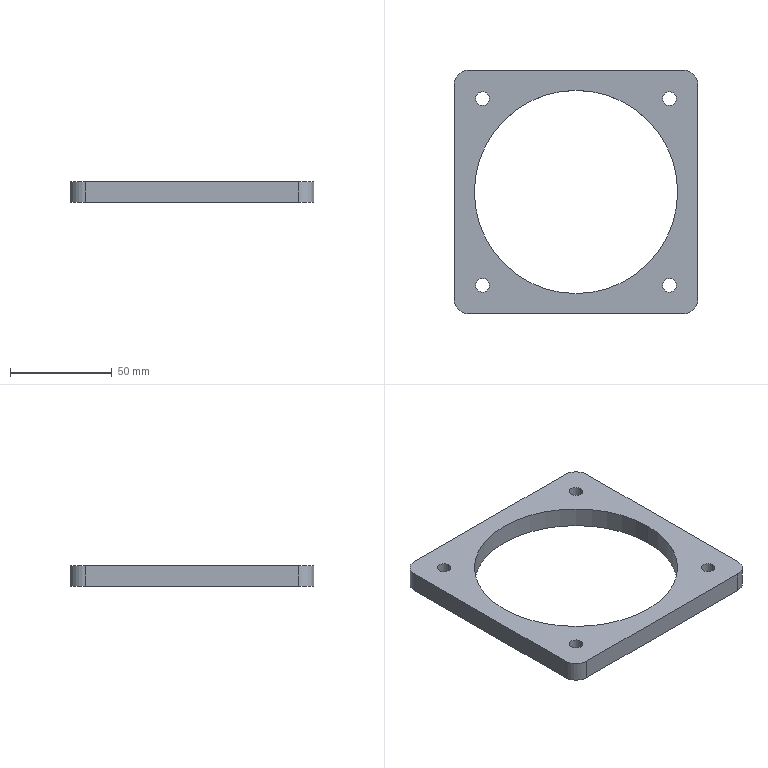Part | SolidWorks | features HoleWzd 2, Extrusion 1, Fillet 1, ICE 1 | 1 solid | 28 faces | box 120 x 120 x 10 mm | volume 63169 mm3 | cylinder 18 | plane 6 | cone 4 | commonest cylinder face diameters 6.8 x8 4.2 x4 15 x4 100 x2
STEP:
#1=CARTESIAN_POINT('',(-49.362,45.962,0.));
#2=VERTEX_POINT('',#1);
#3=CARTESIAN_POINT('',(-42.562,45.962,0.));
#4=VERTEX_POINT('',#3);
#5=CARTESIAN_POINT('',(-45.962,45.962,0.));
#6=DIRECTION('',(0.,0.,1.));
#7=DIRECTION('',(1.,0.,0.));
#8=AXIS2_PLACEMENT_3D('',#5,#6,#7);
#9=CIRCLE('',#8,3.4);
#10=EDGE_CURVE('',#2,#4,#9,.T.);
#11=ORIENTED_EDGE('',*,*,#10,.F.);
#12=CARTESIAN_POINT('',(-49.362,45.962,10.));
#13=VERTEX_POINT('',#12);
#14=CARTESIAN_POINT('',(-49.362,45.962,10.));
#15=DIRECTION('',(0.,0.,1.));
#16=VECTOR('',#15,1000.);
#17=LINE('',#14,#16);
#18=EDGE_CURVE('',#2,#13,#17,.T.);
#19=ORIENTED_EDGE('',*,*,#18,.T.);
#20=CARTESIAN_POINT('',(-42.562,45.962,10.));
#21=VERTEX_POINT('',#20);
#22=CARTESIAN_POINT('',(-45.962,45.962,10.));
#23=DIRECTION('',(0.,0.,1.));
#24=DIRECTION('',(1.,0.,0.));
#25=AXIS2_PLACEMENT_3D('',#22,#23,#24);
#26=CIRCLE('',#25,3.4);
#27=EDGE_CURVE('',#13,#21,#26,.T.);
#28=ORIENTED_EDGE('',*,*,#27,.T.);
#29=CARTESIAN_POINT('',(-42.562,45.962,10.));
#30=DIRECTION('',(0.,0.,1.));
#31=VECTOR('',#30,1000.);
#32=LINE('',#29,#31);
#33=EDGE_CURVE('',#4,#21,#32,.T.);
#34=ORIENTED_EDGE('',*,*,#33,.F.);
#35=EDGE_LOOP('',(#11,#19,#28,#34));
#36=FACE_OUTER_BOUND('',#35,.T.);
#37=CARTESIAN_POINT('',(-45.962,45.962,10.));
#38=DIRECTION('',(0.,0.,1.));
#39=DIRECTION('',(1.,0.,0.));
#40=AXIS2_PLACEMENT_3D('',#37,#38,#39);
#41=CYLINDRICAL_SURFACE('',#40,3.4);
#42=ADVANCED_FACE('',(#36),#41,.F.);
#43=CARTESIAN_POINT('',(42.562,45.962,0.));
#44=VERTEX_POINT('',#43);
#45=CARTESIAN_POINT('',(49.362,45.962,0.));
#46=VERTEX_POINT('',#45);
#47=CARTESIAN_POINT('',(45.962,45.962,0.));
#48=DIRECTION('',(0.,0.,1.));
#49=DIRECTION('',(1.,0.,0.));
#50=AXIS2_PLACEMENT_3D('',#47,#48,#49);
#51=CIRCLE('',#50,3.4);
#52=EDGE_CURVE('',#44,#46,#51,.T.);
#53=ORIENTED_EDGE('',*,*,#52,.F.);
#54=CARTESIAN_POINT('',(42.562,45.962,10.));
#55=VERTEX_POINT('',#54);
#56=CARTESIAN_POINT('',(42.562,45.962,10.));
#57=DIRECTION('',(0.,0.,1.));
#58=VECTOR('',#57,1000.);
#59=LINE('',#56,#58);
#60=EDGE_CURVE('',#44,#55,#59,.T.);
#61=ORIENTED_EDGE('',*,*,#60,.T.);
#62=CARTESIAN_POINT('',(49.362,45.962,10.));
#63=VERTEX_POINT('',#62);
#64=CARTESIAN_POINT('',(45.962,45.962,10.));
#65=DIRECTION('',(0.,0.,1.));
#66=DIRECTION('',(1.,0.,0.));
#67=AXIS2_PLACEMENT_3D('',#64,#65,#66);
#68=CIRCLE('',#67,3.4);
#69=EDGE_CURVE('',#55,#63,#68,.T.);
#70=ORIENTED_EDGE('',*,*,#69,.T.);
#71=CARTESIAN_POINT('',(49.362,45.962,10.));
#72=DIRECTION('',(0.,0.,1.));
#73=VECTOR('',#72,1000.);
#74=LINE('',#71,#73);
#75=EDGE_CURVE('',#46,#63,#74,.T.);
#76=ORIENTED_EDGE('',*,*,#75,.F.);
#77=EDGE_LOOP('',(#53,#61,#70,#76));
#78=FACE_OUTER_BOUND('',#77,.T.);
#79=CARTESIAN_POINT('',(45.962,45.962,10.));
#80=DIRECTION('',(0.,0.,1.));
#81=DIRECTION('',(1.,0.,0.));
#82=AXIS2_PLACEMENT_3D('',#79,#80,#81);
#83=CYLINDRICAL_SURFACE('',#82,3.4);
#84=ADVANCED_FACE('',(#78),#83,.F.);
#85=CARTESIAN_POINT('',(42.562,-45.962,0.));
#86=VERTEX_POINT('',#85);
#87=CARTESIAN_POINT('',(49.362,-45.962,0.));
#88=VERTEX_POINT('',#87);
#89=CARTESIAN_POINT('',(45.962,-45.962,0.));
#90=DIRECTION('',(0.,0.,1.));
#91=DIRECTION('',(1.,0.,0.));
#92=AXIS2_PLACEMENT_3D('',#89,#90,#91);
#93=CIRCLE('',#92,3.4);
#94=EDGE_CURVE('',#86,#88,#93,.T.);
#95=ORIENTED_EDGE('',*,*,#94,.F.);
#96=CARTESIAN_POINT('',(42.562,-45.962,10.));
#97=VERTEX_POINT('',#96);
#98=CARTESIAN_POINT('',(42.562,-45.962,10.));
#99=DIRECTION('',(0.,0.,1.));
#100=VECTOR('',#99,1000.);
#101=LINE('',#98,#100);
#102=EDGE_CURVE('',#86,#97,#101,.T.);
#103=ORIENTED_EDGE('',*,*,#102,.T.);
#104=CARTESIAN_POINT('',(49.362,-45.962,10.));
#105=VERTEX_POINT('',#104);
#106=CARTESIAN_POINT('',(45.962,-45.962,10.));
#107=DIRECTION('',(0.,0.,1.));
#108=DIRECTION('',(1.,0.,0.));
#109=AXIS2_PLACEMENT_3D('',#106,#107,#108);
#110=CIRCLE('',#109,3.4);
#111=EDGE_CURVE('',#97,#105,#110,.T.);
#112=ORIENTED_EDGE('',*,*,#111,.T.);
#113=CARTESIAN_POINT('',(49.362,-45.962,10.));
#114=DIRECTION('',(0.,0.,1.));
#115=VECTOR('',#114,1000.);
#116=LINE('',#113,#115);
#117=EDGE_CURVE('',#88,#105,#116,.T.);
#118=ORIENTED_EDGE('',*,*,#117,.F.);
#119=EDGE_LOOP('',(#95,#103,#112,#118));
#120=FACE_OUTER_BOUND('',#119,.T.);
#121=CARTESIAN_POINT('',(45.962,-45.962,10.));
#122=DIRECTION('',(0.,0.,1.));
#123=DIRECTION('',(1.,0.,0.));
#124=AXIS2_PLACEMENT_3D('',#121,#122,#123);
#125=CYLINDRICAL_SURFACE('',#124,3.4);
#126=ADVANCED_FACE('',(#120),#125,.F.);
#127=CARTESIAN_POINT('',(-49.362,-45.962,0.));
#128=VERTEX_POINT('',#127);
#129=CARTESIAN_POINT('',(-42.562,-45.962,0.));
#130=VERTEX_POINT('',#129);
#131=CARTESIAN_POINT('',(-45.962,-45.962,0.));
#132=DIRECTION('',(0.,0.,1.));
#133=DIRECTION('',(1.,0.,0.));
#134=AXIS2_PLACEMENT_3D('',#131,#132,#133);
#135=CIRCLE('',#134,3.4);
#136=EDGE_CURVE('',#128,#130,#135,.T.);
#137=ORIENTED_EDGE('',*,*,#136,.F.);
#138=CARTESIAN_POINT('',(-49.362,-45.962,10.));
#139=VERTEX_POINT('',#138);
#140=CARTESIAN_POINT('',(-49.362,-45.962,10.));
#141=DIRECTION('',(0.,0.,1.));
#142=VECTOR('',#141,1000.);
#143=LINE('',#140,#142);
#144=EDGE_CURVE('',#128,#139,#143,.T.);
#145=ORIENTED_EDGE('',*,*,#144,.T.);
#146=CARTESIAN_POINT('',(-42.562,-45.962,10.));
#147=VERTEX_POINT('',#146);
#148=CARTESIAN_POINT('',(-45.962,-45.962,10.));
#149=DIRECTION('',(0.,0.,1.));
#150=DIRECTION('',(1.,0.,0.));
#151=AXIS2_PLACEMENT_3D('',#148,#149,#150);
#152=CIRCLE('',#151,3.4);
#153=EDGE_CURVE('',#139,#147,#152,.T.);
#154=ORIENTED_EDGE('',*,*,#153,.T.);
#155=CARTESIAN_POINT('',(-42.562,-45.962,10.));
#156=DIRECTION('',(0.,0.,1.));
#157=VECTOR('',#156,1000.);
#158=LINE('',#155,#157);
#159=EDGE_CURVE('',#130,#147,#158,.T.);
#160=ORIENTED_EDGE('',*,*,#159,.F.);
#161=EDGE_LOOP('',(#137,#145,#154,#160));
#162=FACE_OUTER_BOUND('',#161,.T.);
#163=CARTESIAN_POINT('',(-45.962,-45.962,10.));
#164=DIRECTION('',(0.,0.,1.));
#165=DIRECTION('',(1.,0.,0.));
#166=AXIS2_PLACEMENT_3D('',#163,#164,#165);
#167=CYLINDRICAL_SURFACE('',#166,3.4);
#168=ADVANCED_FACE('',(#162),#167,.F.);
#169=CARTESIAN_POINT('',(-50.,0.,0.));
#170=VERTEX_POINT('',#169);
#171=CARTESIAN_POINT('',(50.,0.,0.));
#172=VERTEX_POINT('',#171);
#173=CARTESIAN_POINT('',(0.,0.,0.));
#174=DIRECTION('',(0.,0.,1.));
#175=DIRECTION('',(1.,0.,0.));
#176=AXIS2_PLACEMENT_3D('',#173,#174,#175);
#177=CIRCLE('',#176,50.);
#178=EDGE_CURVE('',#170,#172,#177,.T.);
#179=ORIENTED_EDGE('',*,*,#178,.F.);
#180=CARTESIAN_POINT('',(-50.,0.,10.));
#181=VERTEX_POINT('',#180);
#182=CARTESIAN_POINT('',(-50.,0.,0.));
#183=DIRECTION('',(0.,0.,1.));
#184=VECTOR('',#183,1000.);
#185=LINE('',#182,#184);
#186=EDGE_CURVE('',#170,#181,#185,.T.);
#187=ORIENTED_EDGE('',*,*,#186,.T.);
#188=CARTESIAN_POINT('',(50.,0.,10.));
#189=VERTEX_POINT('',#188);
#190=CARTESIAN_POINT('',(0.,0.,10.));
#191=DIRECTION('',(0.,0.,1.));
#192=DIRECTION('',(1.,0.,0.));
#193=AXIS2_PLACEMENT_3D('',#190,#191,#192);
#194=CIRCLE('',#193,50.);
#195=EDGE_CURVE('',#181,#189,#194,.T.);
#196=ORIENTED_EDGE('',*,*,#195,.T.);
#197=CARTESIAN_POINT('',(50.,0.,0.));
#198=DIRECTION('',(0.,0.,1.));
#199=VECTOR('',#198,1000.);
#200=LINE('',#197,#199);
#201=EDGE_CURVE('',#172,#189,#200,.T.);
#202=ORIENTED_EDGE('',*,*,#201,.F.);
#203=EDGE_LOOP('',(#179,#187,#196,#202));
#204=FACE_OUTER_BOUND('',#203,.T.);
#205=CARTESIAN_POINT('',(0.,0.,0.));
#206=DIRECTION('',(0.,0.,1.));
#207=DIRECTION('',(1.,0.,0.));
#208=AXIS2_PLACEMENT_3D('',#205,#206,#207);
#209=CYLINDRICAL_SURFACE('',#208,50.);
#210=ADVANCED_FACE('',(#204),#209,.F.);
#211=CARTESIAN_POINT('',(-25.,47.6,2.9));
#212=VERTEX_POINT('',#211);
#213=CARTESIAN_POINT('',(-25.,47.6,7.1));
#214=VERTEX_POINT('',#213);
#215=CARTESIAN_POINT('',(-25.,47.6,5.));
#216=DIRECTION('',(0.,1.,0.));
#217=DIRECTION('',(0.,0.,1.));
#218=AXIS2_PLACEMENT_3D('',#215,#216,#217);
#219=CIRCLE('',#218,2.1);
#220=EDGE_CURVE('',#212,#214,#219,.T.);
#221=ORIENTED_EDGE('',*,*,#220,.F.);
#222=CARTESIAN_POINT('',(-25.,60.,2.9));
#223=VERTEX_POINT('',#222);
#224=CARTESIAN_POINT('',(-25.,60.,2.9));
#225=DIRECTION('',(0.,1.,0.));
#226=VECTOR('',#225,1000.);
#227=LINE('',#224,#226);
#228=EDGE_CURVE('',#212,#223,#227,.T.);
#229=ORIENTED_EDGE('',*,*,#228,.T.);
#230=CARTESIAN_POINT('',(-25.,60.,7.1));
#231=VERTEX_POINT('',#230);
#232=CARTESIAN_POINT('',(-25.,60.,5.));
#233=DIRECTION('',(0.,1.,0.));
#234=DIRECTION('',(0.,0.,1.));
#235=AXIS2_PLACEMENT_3D('',#232,#233,#234);
#236=CIRCLE('',#235,2.1);
#237=EDGE_CURVE('',#223,#231,#236,.T.);
#238=ORIENTED_EDGE('',*,*,#237,.T.);
#239=CARTESIAN_POINT('',(-25.,60.,7.1));
#240=DIRECTION('',(0.,1.,0.));
#241=VECTOR('',#240,1000.);
#242=LINE('',#239,#241);
#243=EDGE_CURVE('',#214,#231,#242,.T.);
#244=ORIENTED_EDGE('',*,*,#243,.F.);
#245=EDGE_LOOP('',(#221,#229,#238,#244));
#246=FACE_OUTER_BOUND('',#245,.T.);
#247=CARTESIAN_POINT('',(-25.,60.,5.));
#248=DIRECTION('',(0.,1.,0.));
#249=DIRECTION('',(0.,0.,1.));
#250=AXIS2_PLACEMENT_3D('',#247,#248,#249);
#251=CYLINDRICAL_SURFACE('',#250,2.1);
#252=ADVANCED_FACE('',(#246),#251,.F.);
#253=CARTESIAN_POINT('',(-25.,46.338,5.));
#254=VERTEX_POINT('',#253);
#255=CARTESIAN_POINT('',(-25.,47.6,7.1));
#256=DIRECTION('',(0.,0.515,0.8572));
#257=VECTOR('',#256,1000.);
#258=LINE('',#255,#257);
#259=EDGE_CURVE('',#254,#214,#258,.T.);
#260=ORIENTED_EDGE('',*,*,#259,.F.);
#261=CARTESIAN_POINT('',(-25.,47.6,2.9));
#262=DIRECTION('',(0.,0.515,-0.8572));
#263=VECTOR('',#262,1000.);
#264=LINE('',#261,#263);
#265=EDGE_CURVE('',#254,#212,#264,.T.);
#266=ORIENTED_EDGE('',*,*,#265,.T.);
#267=ORIENTED_EDGE('',*,*,#220,.T.);
#268=EDGE_LOOP('',(#260,#266,#267));
#269=FACE_OUTER_BOUND('',#268,.T.);
#270=CARTESIAN_POINT('',(-25.,47.6,5.));
#271=DIRECTION('',(0.,1.,0.));
#272=DIRECTION('',(0.,0.,1.));
#273=AXIS2_PLACEMENT_3D('',#270,#271,#272);
#274=CONICAL_SURFACE('',#273,2.1,1.03);
#275=ADVANCED_FACE('',(#269),#274,.F.);
#276=CARTESIAN_POINT('',(25.,47.6,2.9));
#277=VERTEX_POINT('',#276);
#278=CARTESIAN_POINT('',(25.,47.6,7.1));
#279=VERTEX_POINT('',#278);
#280=CARTESIAN_POINT('',(25.,47.6,5.));
#281=DIRECTION('',(0.,1.,0.));
#282=DIRECTION('',(0.,0.,1.));
#283=AXIS2_PLACEMENT_3D('',#280,#281,#282);
#284=CIRCLE('',#283,2.1);
#285=EDGE_CURVE('',#277,#279,#284,.T.);
#286=ORIENTED_EDGE('',*,*,#285,.F.);
#287=CARTESIAN_POINT('',(25.,60.,2.9));
#288=VERTEX_POINT('',#287);
#289=CARTESIAN_POINT('',(25.,60.,2.9));
#290=DIRECTION('',(0.,1.,0.));
#291=VECTOR('',#290,1000.);
#292=LINE('',#289,#291);
#293=EDGE_CURVE('',#277,#288,#292,.T.);
#294=ORIENTED_EDGE('',*,*,#293,.T.);
#295=CARTESIAN_POINT('',(25.,60.,7.1));
#296=VERTEX_POINT('',#295);
#297=CARTESIAN_POINT('',(25.,60.,5.));
#298=DIRECTION('',(0.,1.,0.));
#299=DIRECTION('',(0.,0.,1.));
#300=AXIS2_PLACEMENT_3D('',#297,#298,#299);
#301=CIRCLE('',#300,2.1);
#302=EDGE_CURVE('',#288,#296,#301,.T.);
#303=ORIENTED_EDGE('',*,*,#302,.T.);
#304=CARTESIAN_POINT('',(25.,60.,7.1));
#305=DIRECTION('',(0.,1.,0.));
#306=VECTOR('',#305,1000.);
#307=LINE('',#304,#306);
#308=EDGE_CURVE('',#279,#296,#307,.T.);
#309=ORIENTED_EDGE('',*,*,#308,.F.);
#310=EDGE_LOOP('',(#286,#294,#303,#309));
#311=FACE_OUTER_BOUND('',#310,.T.);
#312=CARTESIAN_POINT('',(25.,60.,5.));
#313=DIRECTION('',(0.,1.,0.));
#314=DIRECTION('',(0.,0.,1.));
#315=AXIS2_PLACEMENT_3D('',#312,#313,#314);
#316=CYLINDRICAL_SURFACE('',#315,2.1);
#317=ADVANCED_FACE('',(#311),#316,.F.);
#318=CARTESIAN_POINT('',(25.,46.338,5.));
#319=VERTEX_POINT('',#318);
#320=CARTESIAN_POINT('',(25.,47.6,7.1));
#321=DIRECTION('',(0.,0.515,0.8572));
#322=VECTOR('',#321,1000.);
#323=LINE('',#320,#322);
#324=EDGE_CURVE('',#319,#279,#323,.T.);
#325=ORIENTED_EDGE('',*,*,#324,.F.);
#326=CARTESIAN_POINT('',(25.,47.6,2.9));
#327=DIRECTION('',(0.,0.515,-0.8572));
#328=VECTOR('',#327,1000.);
#329=LINE('',#326,#328);
#330=EDGE_CURVE('',#319,#277,#329,.T.);
#331=ORIENTED_EDGE('',*,*,#330,.T.);
#332=ORIENTED_EDGE('',*,*,#285,.T.);
#333=EDGE_LOOP('',(#325,#331,#332));
#334=FACE_OUTER_BOUND('',#333,.T.);
#335=CARTESIAN_POINT('',(25.,47.6,5.));
#336=DIRECTION('',(0.,1.,0.));
#337=DIRECTION('',(0.,0.,1.));
#338=AXIS2_PLACEMENT_3D('',#335,#336,#337);
#339=CONICAL_SURFACE('',#338,2.1,1.03);
#340=ADVANCED_FACE('',(#334),#339,.F.);
#341=CARTESIAN_POINT('',(-60.,52.5,0.));
#342=VERTEX_POINT('',#341);
#343=CARTESIAN_POINT('',(-60.,-52.5,0.));
#344=VERTEX_POINT('',#343);
#345=CARTESIAN_POINT('',(-60.,-60.,0.));
#346=DIRECTION('',(0.,-1.,0.));
#347=VECTOR('',#346,1000.);
#348=LINE('',#345,#347);
#349=EDGE_CURVE('',#342,#344,#348,.T.);
#350=ORIENTED_EDGE('',*,*,#349,.T.);
#351=CARTESIAN_POINT('',(-60.,-52.5,10.));
#352=VERTEX_POINT('',#351);
#353=CARTESIAN_POINT('',(-60.,-52.5,10.));
#354=DIRECTION('',(0.,0.,1.));
#355=VECTOR('',#354,1000.);
#356=LINE('',#353,#355);
#357=EDGE_CURVE('',#344,#352,#356,.T.);
#358=ORIENTED_EDGE('',*,*,#357,.T.);
#359=CARTESIAN_POINT('',(-60.,52.5,10.));
#360=VERTEX_POINT('',#359);
#361=CARTESIAN_POINT('',(-60.,-60.,10.));
#362=DIRECTION('',(0.,-1.,0.));
#363=VECTOR('',#362,1000.);
#364=LINE('',#361,#363);
#365=EDGE_CURVE('',#360,#352,#364,.T.);
#366=ORIENTED_EDGE('',*,*,#365,.F.);
#367=CARTESIAN_POINT('',(-60.,52.5,10.));
#368=DIRECTION('',(0.,0.,-1.));
#369=VECTOR('',#368,1000.);
#370=LINE('',#367,#369);
#371=EDGE_CURVE('',#360,#342,#370,.T.);
#372=ORIENTED_EDGE('',*,*,#371,.T.);
#373=EDGE_LOOP('',(#350,#358,#366,#372));
#374=FACE_OUTER_BOUND('',#373,.T.);
#375=CARTESIAN_POINT('',(-60.,-60.,10.));
#376=DIRECTION('',(1.,0.,0.));
#377=DIRECTION('',(0.,0.,-1.));
#378=AXIS2_PLACEMENT_3D('',#375,#376,#377);
#379=PLANE('',#378);
#380=ADVANCED_FACE('',(#374),#379,.F.);
#381=CARTESIAN_POINT('',(-52.5,-60.,10.));
#382=VERTEX_POINT('',#381);
#383=CARTESIAN_POINT('',(52.5,-60.,10.));
#384=VERTEX_POINT('',#383);
#385=CARTESIAN_POINT('',(60.,-60.,10.));
#386=DIRECTION('',(1.,0.,0.));
#387=VECTOR('',#386,1000.);
#388=LINE('',#385,#387);
#389=EDGE_CURVE('',#382,#384,#388,.T.);
#390=ORIENTED_EDGE('',*,*,#389,.F.);
#391=CARTESIAN_POINT('',(-52.5,-60.,0.));
#392=VERTEX_POINT('',#391);
#393=CARTESIAN_POINT('',(-52.5,-60.,10.));
#394=DIRECTION('',(0.,0.,-1.));
#395=VECTOR('',#394,1000.);
#396=LINE('',#393,#395);
#397=EDGE_CURVE('',#382,#392,#396,.T.);
#398=ORIENTED_EDGE('',*,*,#397,.T.);
#399=CARTESIAN_POINT('',(52.5,-60.,0.));
#400=VERTEX_POINT('',#399);
#401=CARTESIAN_POINT('',(60.,-60.,0.));
#402=DIRECTION('',(1.,0.,0.));
#403=VECTOR('',#402,1000.);
#404=LINE('',#401,#403);
#405=EDGE_CURVE('',#392,#400,#404,.T.);
#406=ORIENTED_EDGE('',*,*,#405,.T.);
#407=CARTESIAN_POINT('',(52.5,-60.,10.));
#408=DIRECTION('',(0.,0.,1.));
#409=VECTOR('',#408,1000.);
#410=LINE('',#407,#409);
#411=EDGE_CURVE('',#400,#384,#410,.T.);
#412=ORIENTED_EDGE('',*,*,#411,.T.);
#413=EDGE_LOOP('',(#390,#398,#406,#412));
#414=FACE_OUTER_BOUND('',#413,.T.);
#415=CARTESIAN_POINT('',(60.,-60.,10.));
#416=DIRECTION('',(0.,1.,0.));
#417=DIRECTION('',(-1.,0.,0.));
#418=AXIS2_PLACEMENT_3D('',#415,#416,#417);
#419=PLANE('',#418);
#420=ADVANCED_FACE('',(#414),#419,.F.);
#421=CARTESIAN_POINT('',(60.,-52.5,10.));
#422=VERTEX_POINT('',#421);
#423=CARTESIAN_POINT('',(60.,52.5,10.));
#424=VERTEX_POINT('',#423);
#425=CARTESIAN_POINT('',(60.,-60.,10.));
#426=DIRECTION('',(0.,1.,0.));
#427=VECTOR('',#426,1000.);
#428=LINE('',#425,#427);
#429=EDGE_CURVE('',#422,#424,#428,.T.);
#430=ORIENTED_EDGE('',*,*,#429,.F.);
#431=CARTESIAN_POINT('',(60.,-52.5,0.));
#432=VERTEX_POINT('',#431);
#433=CARTESIAN_POINT('',(60.,-52.5,10.));
#434=DIRECTION('',(0.,0.,-1.));
#435=VECTOR('',#434,1000.);
#436=LINE('',#433,#435);
#437=EDGE_CURVE('',#422,#432,#436,.T.);
#438=ORIENTED_EDGE('',*,*,#437,.T.);
#439=CARTESIAN_POINT('',(60.,52.5,0.));
#440=VERTEX_POINT('',#439);
#441=CARTESIAN_POINT('',(60.,-60.,0.));
#442=DIRECTION('',(0.,1.,0.));
#443=VECTOR('',#442,1000.);
#444=LINE('',#441,#443);
#445=EDGE_CURVE('',#432,#440,#444,.T.);
#446=ORIENTED_EDGE('',*,*,#445,.T.);
#447=CARTESIAN_POINT('',(60.,52.5,10.));
#448=DIRECTION('',(0.,0.,1.));
#449=VECTOR('',#448,1000.);
#450=LINE('',#447,#449);
#451=EDGE_CURVE('',#440,#424,#450,.T.);
#452=ORIENTED_EDGE('',*,*,#451,.T.);
#453=EDGE_LOOP('',(#430,#438,#446,#452));
#454=FACE_OUTER_BOUND('',#453,.T.);
#455=CARTESIAN_POINT('',(60.,-60.,10.));
#456=DIRECTION('',(-1.,0.,0.));
#457=DIRECTION('',(0.,-1.,0.));
#458=AXIS2_PLACEMENT_3D('',#455,#456,#457);
#459=PLANE('',#458);
#460=ADVANCED_FACE('',(#454),#459,.F.);
#461=CARTESIAN_POINT('',(-25.,60.,5.));
#462=DIRECTION('',(0.,1.,0.));
#463=DIRECTION('',(0.,0.,1.));
#464=AXIS2_PLACEMENT_3D('',#461,#462,#463);
#465=CIRCLE('',#464,2.1);
#466=EDGE_CURVE('',#231,#223,#465,.T.);
#467=ORIENTED_EDGE('',*,*,#466,.F.);
#468=ORIENTED_EDGE('',*,*,#237,.F.);
#469=EDGE_LOOP('',(#467,#468));
#470=FACE_BOUND('',#469,.T.);
#471=CARTESIAN_POINT('',(25.,60.,5.));
#472=DIRECTION('',(0.,1.,0.));
#473=DIRECTION('',(0.,0.,1.));
#474=AXIS2_PLACEMENT_3D('',#471,#472,#473);
#475=CIRCLE('',#474,2.1);
#476=EDGE_CURVE('',#296,#288,#475,.T.);
#477=ORIENTED_EDGE('',*,*,#476,.F.);
#478=ORIENTED_EDGE('',*,*,#302,.F.);
#479=EDGE_LOOP('',(#477,#478));
#480=FACE_BOUND('',#479,.T.);
#481=CARTESIAN_POINT('',(52.5,60.,10.));
#482=VERTEX_POINT('',#481);
#483=CARTESIAN_POINT('',(-52.5,60.,10.));
#484=VERTEX_POINT('',#483);
#485=CARTESIAN_POINT('',(60.,60.,10.));
#486=DIRECTION('',(-1.,0.,0.));
#487=VECTOR('',#486,1000.);
#488=LINE('',#485,#487);
#489=EDGE_CURVE('',#482,#484,#488,.T.);
#490=ORIENTED_EDGE('',*,*,#489,.F.);
#491=CARTESIAN_POINT('',(52.5,60.,0.));
#492=VERTEX_POINT('',#491);
#493=CARTESIAN_POINT('',(52.5,60.,10.));
#494=DIRECTION('',(0.,0.,-1.));
#495=VECTOR('',#494,1000.);
#496=LINE('',#493,#495);
#497=EDGE_CURVE('',#482,#492,#496,.T.);
#498=ORIENTED_EDGE('',*,*,#497,.T.);
#499=CARTESIAN_POINT('',(-52.5,60.,0.));
#500=VERTEX_POINT('',#499);
#501=CARTESIAN_POINT('',(60.,60.,0.));
#502=DIRECTION('',(-1.,0.,0.));
#503=VECTOR('',#502,1000.);
#504=LINE('',#501,#503);
#505=EDGE_CURVE('',#492,#500,#504,.T.);
#506=ORIENTED_EDGE('',*,*,#505,.T.);
#507=CARTESIAN_POINT('',(-52.5,60.,10.));
#508=DIRECTION('',(0.,0.,1.));
#509=VECTOR('',#508,1000.);
#510=LINE('',#507,#509);
#511=EDGE_CURVE('',#500,#484,#510,.T.);
#512=ORIENTED_EDGE('',*,*,#511,.T.);
#513=EDGE_LOOP('',(#490,#498,#506,#512));
#514=FACE_OUTER_BOUND('',#513,.T.);
#515=CARTESIAN_POINT('',(60.,60.,10.));
#516=DIRECTION('',(0.,-1.,0.));
#517=DIRECTION('',(1.,0.,0.));
#518=AXIS2_PLACEMENT_3D('',#515,#516,#517);
#519=PLANE('',#518);
#520=ADVANCED_FACE('',(#470,#480,#514),#519,.F.);
#521=CARTESIAN_POINT('',(-45.962,45.962,10.));
#522=DIRECTION('',(0.,0.,1.));
#523=DIRECTION('',(1.,0.,0.));
#524=AXIS2_PLACEMENT_3D('',#521,#522,#523);
#525=CIRCLE('',#524,3.4);
#526=EDGE_CURVE('',#21,#13,#525,.T.);
#527=ORIENTED_EDGE('',*,*,#526,.F.);
#528=ORIENTED_EDGE('',*,*,#27,.F.);
#529=EDGE_LOOP('',(#527,#528));
#530=FACE_BOUND('',#529,.T.);
#531=CARTESIAN_POINT('',(45.962,45.962,10.));
#532=DIRECTION('',(0.,0.,1.));
#533=DIRECTION('',(1.,0.,0.));
#534=AXIS2_PLACEMENT_3D('',#531,#532,#533);
#535=CIRCLE('',#534,3.4);
#536=EDGE_CURVE('',#63,#55,#535,.T.);
#537=ORIENTED_EDGE('',*,*,#536,.F.);
#538=ORIENTED_EDGE('',*,*,#69,.F.);
#539=EDGE_LOOP('',(#537,#538));
#540=FACE_BOUND('',#539,.T.);
#541=CARTESIAN_POINT('',(45.962,-45.962,10.));
#542=DIRECTION('',(0.,0.,1.));
#543=DIRECTION('',(1.,0.,0.));
#544=AXIS2_PLACEMENT_3D('',#541,#542,#543);
#545=CIRCLE('',#544,3.4);
#546=EDGE_CURVE('',#105,#97,#545,.T.);
#547=ORIENTED_EDGE('',*,*,#546,.F.);
#548=ORIENTED_EDGE('',*,*,#111,.F.);
#549=EDGE_LOOP('',(#547,#548));
#550=FACE_BOUND('',#549,.T.);
#551=CARTESIAN_POINT('',(-45.962,-45.962,10.));
#552=DIRECTION('',(0.,0.,1.));
#553=DIRECTION('',(1.,0.,0.));
#554=AXIS2_PLACEMENT_3D('',#551,#552,#553);
#555=CIRCLE('',#554,3.4);
#556=EDGE_CURVE('',#147,#139,#555,.T.);
#557=ORIENTED_EDGE('',*,*,#556,.F.);
#558=ORIENTED_EDGE('',*,*,#153,.F.);
#559=EDGE_LOOP('',(#557,#558));
#560=FACE_BOUND('',#559,.T.);
#561=CARTESIAN_POINT('',(0.,0.,10.));
#562=DIRECTION('',(0.,0.,1.));
#563=DIRECTION('',(1.,0.,0.));
#564=AXIS2_PLACEMENT_3D('',#561,#562,#563);
#565=CIRCLE('',#564,50.);
#566=EDGE_CURVE('',#189,#181,#565,.T.);
#567=ORIENTED_EDGE('',*,*,#566,.F.);
#568=ORIENTED_EDGE('',*,*,#195,.F.);
#569=EDGE_LOOP('',(#567,#568));
#570=FACE_BOUND('',#569,.T.);
#571=ORIENTED_EDGE('',*,*,#365,.T.);
#572=CARTESIAN_POINT('',(-52.5,-52.5,10.));
#573=DIRECTION('',(0.,0.,1.));
#574=DIRECTION('',(1.,0.,0.));
#575=AXIS2_PLACEMENT_3D('',#572,#573,#574);
#576=CIRCLE('',#575,7.5);
#577=EDGE_CURVE('',#352,#382,#576,.T.);
#578=ORIENTED_EDGE('',*,*,#577,.T.);
#579=ORIENTED_EDGE('',*,*,#389,.T.);
#580=CARTESIAN_POINT('',(52.5,-52.5,10.));
#581=DIRECTION('',(0.,0.,1.));
#582=DIRECTION('',(1.,0.,0.));
#583=AXIS2_PLACEMENT_3D('',#580,#581,#582);
#584=CIRCLE('',#583,7.5);
#585=EDGE_CURVE('',#384,#422,#584,.T.);
#586=ORIENTED_EDGE('',*,*,#585,.T.);
#587=ORIENTED_EDGE('',*,*,#429,.T.);
#588=CARTESIAN_POINT('',(52.5,52.5,10.));
#589=DIRECTION('',(0.,0.,1.));
#590=DIRECTION('',(1.,0.,0.));
#591=AXIS2_PLACEMENT_3D('',#588,#589,#590);
#592=CIRCLE('',#591,7.5);
#593=EDGE_CURVE('',#424,#482,#592,.T.);
#594=ORIENTED_EDGE('',*,*,#593,.T.);
#595=ORIENTED_EDGE('',*,*,#489,.T.);
#596=CARTESIAN_POINT('',(-52.5,52.5,10.));
#597=DIRECTION('',(0.,0.,1.));
#598=DIRECTION('',(1.,0.,0.));
#599=AXIS2_PLACEMENT_3D('',#596,#597,#598);
#600=CIRCLE('',#599,7.5);
#601=EDGE_CURVE('',#484,#360,#600,.T.);
#602=ORIENTED_EDGE('',*,*,#601,.T.);
#603=EDGE_LOOP('',(#571,#578,#579,#586,#587,#594,#595,#602));
#604=FACE_OUTER_BOUND('',#603,.T.);
#605=CARTESIAN_POINT('',(0.,0.,10.));
#606=DIRECTION('',(0.,0.,1.));
#607=DIRECTION('',(1.,0.,0.));
#608=AXIS2_PLACEMENT_3D('',#605,#606,#607);
#609=PLANE('',#608);
#610=ADVANCED_FACE('',(#530,#540,#550,#560,#570,#604),#609,.T.);
#611=CARTESIAN_POINT('',(-45.962,45.962,0.));
#612=DIRECTION('',(0.,0.,1.));
#613=DIRECTION('',(1.,0.,0.));
#614=AXIS2_PLACEMENT_3D('',#611,#612,#613);
#615=CIRCLE('',#614,3.4);
#616=EDGE_CURVE('',#4,#2,#615,.T.);
#617=ORIENTED_EDGE('',*,*,#616,.T.);
#618=ORIENTED_EDGE('',*,*,#10,.T.);
#619=EDGE_LOOP('',(#617,#618));
#620=FACE_BOUND('',#619,.T.);
#621=CARTESIAN_POINT('',(45.962,45.962,0.));
#622=DIRECTION('',(0.,0.,1.));
#623=DIRECTION('',(1.,0.,0.));
#624=AXIS2_PLACEMENT_3D('',#621,#622,#623);
#625=CIRCLE('',#624,3.4);
#626=EDGE_CURVE('',#46,#44,#625,.T.);
#627=ORIENTED_EDGE('',*,*,#626,.T.);
#628=ORIENTED_EDGE('',*,*,#52,.T.);
#629=EDGE_LOOP('',(#627,#628));
#630=FACE_BOUND('',#629,.T.);
#631=CARTESIAN_POINT('',(45.962,-45.962,0.));
#632=DIRECTION('',(0.,0.,1.));
#633=DIRECTION('',(1.,0.,0.));
#634=AXIS2_PLACEMENT_3D('',#631,#632,#633);
#635=CIRCLE('',#634,3.4);
#636=EDGE_CURVE('',#88,#86,#635,.T.);
#637=ORIENTED_EDGE('',*,*,#636,.T.);
#638=ORIENTED_EDGE('',*,*,#94,.T.);
#639=EDGE_LOOP('',(#637,#638));
#640=FACE_BOUND('',#639,.T.);
#641=CARTESIAN_POINT('',(-45.962,-45.962,0.));
#642=DIRECTION('',(0.,0.,1.));
#643=DIRECTION('',(1.,0.,0.));
#644=AXIS2_PLACEMENT_3D('',#641,#642,#643);
#645=CIRCLE('',#644,3.4);
#646=EDGE_CURVE('',#130,#128,#645,.T.);
#647=ORIENTED_EDGE('',*,*,#646,.T.);
#648=ORIENTED_EDGE('',*,*,#136,.T.);
#649=EDGE_LOOP('',(#647,#648));
#650=FACE_BOUND('',#649,.T.);
#651=CARTESIAN_POINT('',(0.,0.,0.));
#652=DIRECTION('',(0.,0.,1.));
#653=DIRECTION('',(1.,0.,0.));
#654=AXIS2_PLACEMENT_3D('',#651,#652,#653);
#655=CIRCLE('',#654,50.);
#656=EDGE_CURVE('',#172,#170,#655,.T.);
#657=ORIENTED_EDGE('',*,*,#656,.T.);
#658=ORIENTED_EDGE('',*,*,#178,.T.);
#659=EDGE_LOOP('',(#657,#658));
#660=FACE_BOUND('',#659,.T.);
#661=ORIENTED_EDGE('',*,*,#405,.F.);
#662=CARTESIAN_POINT('',(-52.5,-52.5,0.));
#663=DIRECTION('',(0.,0.,-1.));
#664=DIRECTION('',(1.,0.,0.));
#665=AXIS2_PLACEMENT_3D('',#662,#663,#664);
#666=CIRCLE('',#665,7.5);
#667=EDGE_CURVE('',#392,#344,#666,.T.);
#668=ORIENTED_EDGE('',*,*,#667,.T.);
#669=ORIENTED_EDGE('',*,*,#349,.F.);
#670=CARTESIAN_POINT('',(-52.5,52.5,0.));
#671=DIRECTION('',(0.,0.,-1.));
#672=DIRECTION('',(1.,0.,0.));
#673=AXIS2_PLACEMENT_3D('',#670,#671,#672);
#674=CIRCLE('',#673,7.5);
#675=EDGE_CURVE('',#342,#500,#674,.T.);
#676=ORIENTED_EDGE('',*,*,#675,.T.);
#677=ORIENTED_EDGE('',*,*,#505,.F.);
#678=CARTESIAN_POINT('',(52.5,52.5,0.));
#679=DIRECTION('',(0.,0.,-1.));
#680=DIRECTION('',(1.,0.,0.));
#681=AXIS2_PLACEMENT_3D('',#678,#679,#680);
#682=CIRCLE('',#681,7.5);
#683=EDGE_CURVE('',#492,#440,#682,.T.);
#684=ORIENTED_EDGE('',*,*,#683,.T.);
#685=ORIENTED_EDGE('',*,*,#445,.F.);
#686=CARTESIAN_POINT('',(52.5,-52.5,0.));
#687=DIRECTION('',(0.,0.,-1.));
#688=DIRECTION('',(1.,0.,0.));
#689=AXIS2_PLACEMENT_3D('',#686,#687,#688);
#690=CIRCLE('',#689,7.5);
#691=EDGE_CURVE('',#432,#400,#690,.T.);
#692=ORIENTED_EDGE('',*,*,#691,.T.);
#693=EDGE_LOOP('',(#661,#668,#669,#676,#677,#684,#685,#692));
#694=FACE_OUTER_BOUND('',#693,.T.);
#695=CARTESIAN_POINT('',(0.,0.,0.));
#696=DIRECTION('',(0.,0.,1.));
#697=DIRECTION('',(1.,0.,0.));
#698=AXIS2_PLACEMENT_3D('',#695,#696,#697);
#699=PLANE('',#698);
#700=ADVANCED_FACE('',(#620,#630,#640,#650,#660,#694),#699,.F.);
#701=ORIENTED_EDGE('',*,*,#577,.F.);
#702=ORIENTED_EDGE('',*,*,#357,.F.);
#703=ORIENTED_EDGE('',*,*,#667,.F.);
#704=ORIENTED_EDGE('',*,*,#397,.F.);
#705=EDGE_LOOP('',(#701,#702,#703,#704));
#706=FACE_OUTER_BOUND('',#705,.T.);
#707=CARTESIAN_POINT('',(-52.5,-52.5,10.));
#708=DIRECTION('',(0.,0.,-1.));
#709=DIRECTION('',(-1.,0.,0.));
#710=AXIS2_PLACEMENT_3D('',#707,#708,#709);
#711=CYLINDRICAL_SURFACE('',#710,7.5);
#712=ADVANCED_FACE('',(#706),#711,.T.);
#713=ORIENTED_EDGE('',*,*,#585,.F.);
#714=ORIENTED_EDGE('',*,*,#411,.F.);
#715=ORIENTED_EDGE('',*,*,#691,.F.);
#716=ORIENTED_EDGE('',*,*,#437,.F.);
#717=EDGE_LOOP('',(#713,#714,#715,#716));
#718=FACE_OUTER_BOUND('',#717,.T.);
#719=CARTESIAN_POINT('',(52.5,-52.5,10.));
#720=DIRECTION('',(0.,0.,-1.));
#721=DIRECTION('',(-1.,0.,0.));
#722=AXIS2_PLACEMENT_3D('',#719,#720,#721);
#723=CYLINDRICAL_SURFACE('',#722,7.5);
#724=ADVANCED_FACE('',(#718),#723,.T.);
#725=ORIENTED_EDGE('',*,*,#593,.F.);
#726=ORIENTED_EDGE('',*,*,#451,.F.);
#727=ORIENTED_EDGE('',*,*,#683,.F.);
#728=ORIENTED_EDGE('',*,*,#497,.F.);
#729=EDGE_LOOP('',(#725,#726,#727,#728));
#730=FACE_OUTER_BOUND('',#729,.T.);
#731=CARTESIAN_POINT('',(52.5,52.5,10.));
#732=DIRECTION('',(0.,0.,-1.));
#733=DIRECTION('',(-1.,0.,0.));
#734=AXIS2_PLACEMENT_3D('',#731,#732,#733);
#735=CYLINDRICAL_SURFACE('',#734,7.5);
#736=ADVANCED_FACE('',(#730),#735,.T.);
#737=ORIENTED_EDGE('',*,*,#601,.F.);
#738=ORIENTED_EDGE('',*,*,#511,.F.);
#739=ORIENTED_EDGE('',*,*,#675,.F.);
#740=ORIENTED_EDGE('',*,*,#371,.F.);
#741=EDGE_LOOP('',(#737,#738,#739,#740));
#742=FACE_OUTER_BOUND('',#741,.T.);
#743=CARTESIAN_POINT('',(-52.5,52.5,10.));
#744=DIRECTION('',(0.,0.,-1.));
#745=DIRECTION('',(-1.,0.,0.));
#746=AXIS2_PLACEMENT_3D('',#743,#744,#745);
#747=CYLINDRICAL_SURFACE('',#746,7.5);
#748=ADVANCED_FACE('',(#742),#747,.T.);
#749=ORIENTED_EDGE('',*,*,#330,.F.);
#750=ORIENTED_EDGE('',*,*,#324,.T.);
#751=CARTESIAN_POINT('',(25.,47.6,5.));
#752=DIRECTION('',(0.,1.,0.));
#753=DIRECTION('',(0.,0.,1.));
#754=AXIS2_PLACEMENT_3D('',#751,#752,#753);
#755=CIRCLE('',#754,2.1);
#756=EDGE_CURVE('',#279,#277,#755,.T.);
#757=ORIENTED_EDGE('',*,*,#756,.T.);
#758=EDGE_LOOP('',(#749,#750,#757));
#759=FACE_OUTER_BOUND('',#758,.T.);
#760=CARTESIAN_POINT('',(25.,47.6,5.));
#761=DIRECTION('',(0.,1.,0.));
#762=DIRECTION('',(0.,0.,1.));
#763=AXIS2_PLACEMENT_3D('',#760,#761,#762);
#764=CONICAL_SURFACE('',#763,2.1,1.03);
#765=ADVANCED_FACE('',(#759),#764,.F.);
#766=ORIENTED_EDGE('',*,*,#293,.F.);
#767=ORIENTED_EDGE('',*,*,#756,.F.);
#768=ORIENTED_EDGE('',*,*,#308,.T.);
#769=ORIENTED_EDGE('',*,*,#476,.T.);
#770=EDGE_LOOP('',(#766,#767,#768,#769));
#771=FACE_OUTER_BOUND('',#770,.T.);
#772=CARTESIAN_POINT('',(25.,60.,5.));
#773=DIRECTION('',(0.,1.,0.));
#774=DIRECTION('',(0.,0.,1.));
#775=AXIS2_PLACEMENT_3D('',#772,#773,#774);
#776=CYLINDRICAL_SURFACE('',#775,2.1);
#777=ADVANCED_FACE('',(#771),#776,.F.);
#778=ORIENTED_EDGE('',*,*,#265,.F.);
#779=ORIENTED_EDGE('',*,*,#259,.T.);
#780=CARTESIAN_POINT('',(-25.,47.6,5.));
#781=DIRECTION('',(0.,1.,0.));
#782=DIRECTION('',(0.,0.,1.));
#783=AXIS2_PLACEMENT_3D('',#780,#781,#782);
#784=CIRCLE('',#783,2.1);
#785=EDGE_CURVE('',#214,#212,#784,.T.);
#786=ORIENTED_EDGE('',*,*,#785,.T.);
#787=EDGE_LOOP('',(#778,#779,#786));
#788=FACE_OUTER_BOUND('',#787,.T.);
#789=CARTESIAN_POINT('',(-25.,47.6,5.));
#790=DIRECTION('',(0.,1.,0.));
#791=DIRECTION('',(0.,0.,1.));
#792=AXIS2_PLACEMENT_3D('',#789,#790,#791);
#793=CONICAL_SURFACE('',#792,2.1,1.03);
#794=ADVANCED_FACE('',(#788),#793,.F.);
#795=ORIENTED_EDGE('',*,*,#228,.F.);
#796=ORIENTED_EDGE('',*,*,#785,.F.);
#797=ORIENTED_EDGE('',*,*,#243,.T.);
#798=ORIENTED_EDGE('',*,*,#466,.T.);
#799=EDGE_LOOP('',(#795,#796,#797,#798));
#800=FACE_OUTER_BOUND('',#799,.T.);
#801=CARTESIAN_POINT('',(-25.,60.,5.));
#802=DIRECTION('',(0.,1.,0.));
#803=DIRECTION('',(0.,0.,1.));
#804=AXIS2_PLACEMENT_3D('',#801,#802,#803);
#805=CYLINDRICAL_SURFACE('',#804,2.1);
#806=ADVANCED_FACE('',(#800),#805,.F.);
#807=ORIENTED_EDGE('',*,*,#186,.F.);
#808=ORIENTED_EDGE('',*,*,#656,.F.);
#809=ORIENTED_EDGE('',*,*,#201,.T.);
#810=ORIENTED_EDGE('',*,*,#566,.T.);
#811=EDGE_LOOP('',(#807,#808,#809,#810));
#812=FACE_OUTER_BOUND('',#811,.T.);
#813=CARTESIAN_POINT('',(0.,0.,0.));
#814=DIRECTION('',(0.,0.,1.));
#815=DIRECTION('',(1.,0.,0.));
#816=AXIS2_PLACEMENT_3D('',#813,#814,#815);
#817=CYLINDRICAL_SURFACE('',#816,50.);
#818=ADVANCED_FACE('',(#812),#817,.F.);
#819=ORIENTED_EDGE('',*,*,#144,.F.);
#820=ORIENTED_EDGE('',*,*,#646,.F.);
#821=ORIENTED_EDGE('',*,*,#159,.T.);
#822=ORIENTED_EDGE('',*,*,#556,.T.);
#823=EDGE_LOOP('',(#819,#820,#821,#822));
#824=FACE_OUTER_BOUND('',#823,.T.);
#825=CARTESIAN_POINT('',(-45.962,-45.962,10.));
#826=DIRECTION('',(0.,0.,1.));
#827=DIRECTION('',(1.,0.,0.));
#828=AXIS2_PLACEMENT_3D('',#825,#826,#827);
#829=CYLINDRICAL_SURFACE('',#828,3.4);
#830=ADVANCED_FACE('',(#824),#829,.F.);
#831=ORIENTED_EDGE('',*,*,#102,.F.);
#832=ORIENTED_EDGE('',*,*,#636,.F.);
#833=ORIENTED_EDGE('',*,*,#117,.T.);
#834=ORIENTED_EDGE('',*,*,#546,.T.);
#835=EDGE_LOOP('',(#831,#832,#833,#834));
#836=FACE_OUTER_BOUND('',#835,.T.);
#837=CARTESIAN_POINT('',(45.962,-45.962,10.));
#838=DIRECTION('',(0.,0.,1.));
#839=DIRECTION('',(1.,0.,0.));
#840=AXIS2_PLACEMENT_3D('',#837,#838,#839);
#841=CYLINDRICAL_SURFACE('',#840,3.4);
#842=ADVANCED_FACE('',(#836),#841,.F.);
#843=ORIENTED_EDGE('',*,*,#60,.F.);
#844=ORIENTED_EDGE('',*,*,#626,.F.);
#845=ORIENTED_EDGE('',*,*,#75,.T.);
#846=ORIENTED_EDGE('',*,*,#536,.T.);
#847=EDGE_LOOP('',(#843,#844,#845,#846));
#848=FACE_OUTER_BOUND('',#847,.T.);
#849=CARTESIAN_POINT('',(45.962,45.962,10.));
#850=DIRECTION('',(0.,0.,1.));
#851=DIRECTION('',(1.,0.,0.));
#852=AXIS2_PLACEMENT_3D('',#849,#850,#851);
#853=CYLINDRICAL_SURFACE('',#852,3.4);
#854=ADVANCED_FACE('',(#848),#853,.F.);
#855=ORIENTED_EDGE('',*,*,#18,.F.);
#856=ORIENTED_EDGE('',*,*,#616,.F.);
#857=ORIENTED_EDGE('',*,*,#33,.T.);
#858=ORIENTED_EDGE('',*,*,#526,.T.);
#859=EDGE_LOOP('',(#855,#856,#857,#858));
#860=FACE_OUTER_BOUND('',#859,.T.);
#861=CARTESIAN_POINT('',(-45.962,45.962,10.));
#862=DIRECTION('',(0.,0.,1.));
#863=DIRECTION('',(1.,0.,0.));
#864=AXIS2_PLACEMENT_3D('',#861,#862,#863);
#865=CYLINDRICAL_SURFACE('',#864,3.4);
#866=ADVANCED_FACE('',(#860),#865,.F.);
#867=CLOSED_SHELL('',(#42,#84,#126,#168,#210,#252,#275,#317,#340,#380,#420,#460,#520,#610,#700,#712,#724,#736,#748,#765,#777,#794,#806,#818,#830,#842,#854,#866));
#868=MANIFOLD_SOLID_BREP('',#867);
#869=CARTESIAN_POINT('',(0.,0.,0.));
#870=DIRECTION('',(0.,0.,1.));
#871=DIRECTION('',(1.,0.,0.));
#872=AXIS2_PLACEMENT_3D('',#869,#870,#871);
#873=(LENGTH_UNIT()NAMED_UNIT(*)SI_UNIT(.MILLI.,.METRE.));
#874=UNCERTAINTY_MEASURE_WITH_UNIT(LENGTH_MEASURE(0.00001),#873,'','');
#875=(NAMED_UNIT(*)PLANE_ANGLE_UNIT()SI_UNIT($,.RADIAN.));
#876=(NAMED_UNIT(*)SI_UNIT($,.STERADIAN.)SOLID_ANGLE_UNIT());
#877=(GEOMETRIC_REPRESENTATION_CONTEXT(3)GLOBAL_UNCERTAINTY_ASSIGNED_CONTEXT((#874))GLOBAL_UNIT_ASSIGNED_CONTEXT((#873,#875,#876))REPRESENTATION_CONTEXT('',''));
#878=ADVANCED_BREP_SHAPE_REPRESENTATION('',(#868,#872),#877);